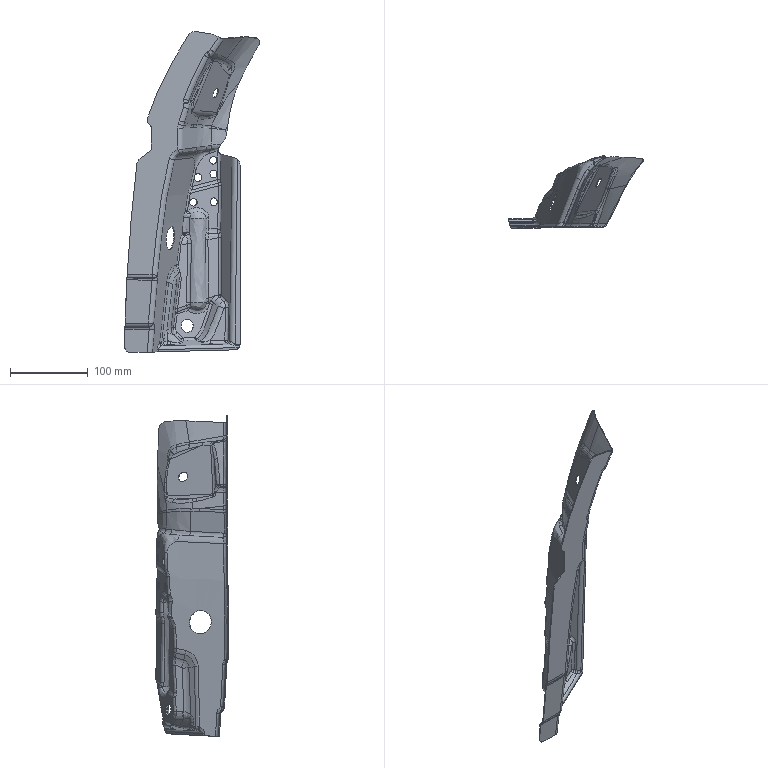Part | STEP file | FNA5401951 | 1 solid | 549 faces | box 173.275 x 92.989 x 412.618 mm | volume 89975 mm3 | spline 392 | cylinder 95 | plane 40 | sphere 12 | other 10 | commonest cylinder face diameters 10 x23 7.6 x11 12 x10 14.4 x6 9.6 x4 21.4 x4